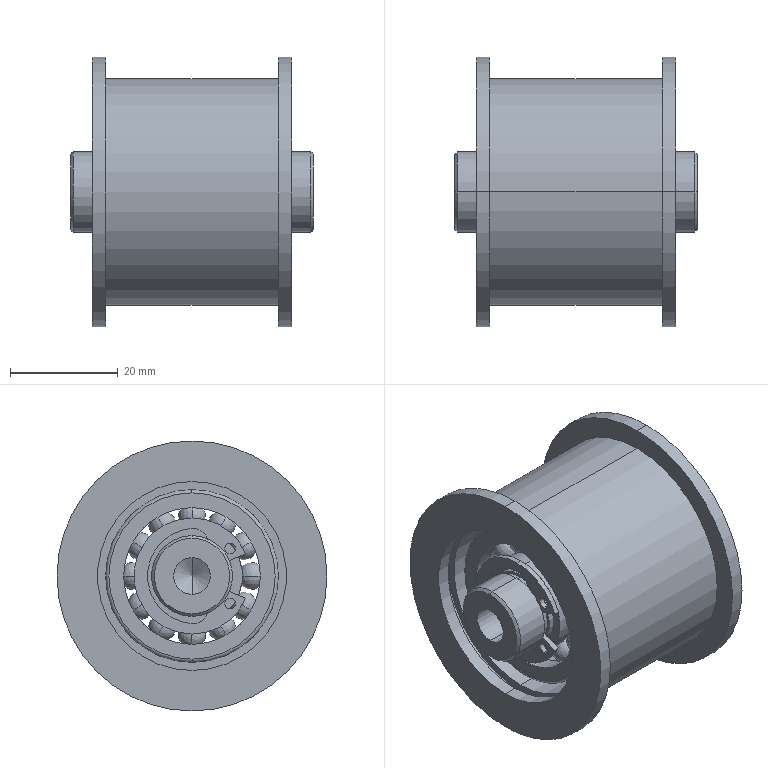Part | SolidWorks | features ReferencePattern 2, AEMSimFeature 1, MirrorCompFeat 1 | 6 solids | 260 faces | box 45 x 50 x 50 mm | volume 36645 mm3 | torus 88 | cylinder 84 | sphere 48 | plane 32 | cone 8 | commonest cylinder face diameters 2 x8 18.667 x8 25.333 x8 35 x8 5.6 x6 15 x6